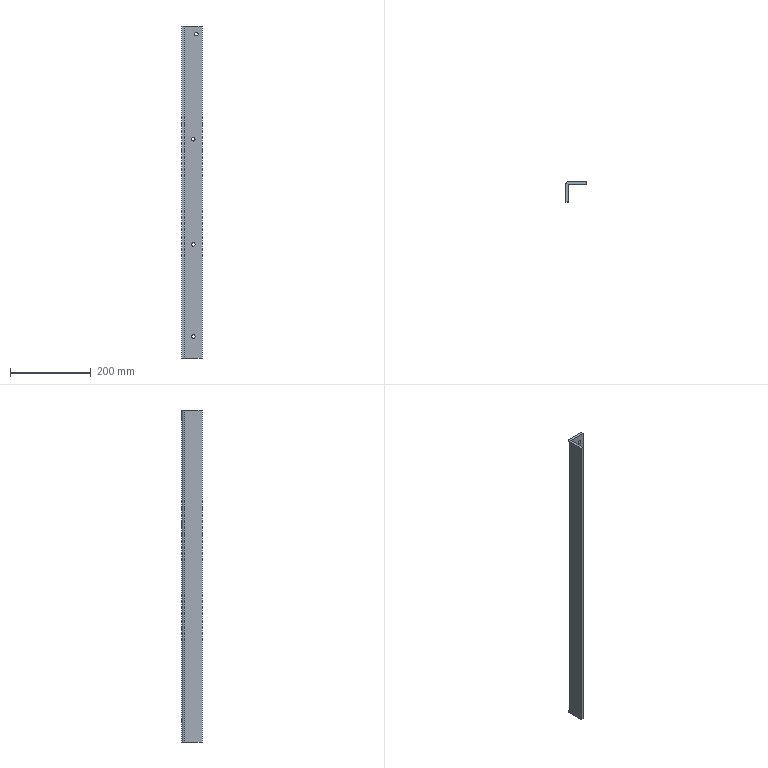Part | SolidWorks | features BaseBody 1 | 1 solid | 18 faces | box 50 x 50 x 821 mm | volume 453617 mm3 | cylinder 10 | plane 8 | commonest cylinder face diameters 9 x8 1.473 x1 13.473 x1
STEP:
#1=CARTESIAN_POINT('',(28.,50.,57.5));
#2=VERTEX_POINT('',#1);
#3=CARTESIAN_POINT('',(28.,50.,48.5));
#4=VERTEX_POINT('',#3);
#5=CARTESIAN_POINT('',(28.,50.,53.));
#6=DIRECTION('',(0.,-1.,0.));
#7=DIRECTION('',(0.,0.,-1.));
#8=AXIS2_PLACEMENT_3D('',#5,#6,#7);
#9=CIRCLE('',#8,4.5);
#10=EDGE_CURVE('',#2,#4,#9,.T.);
#11=ORIENTED_EDGE('',*,*,#10,.F.);
#12=CARTESIAN_POINT('',(28.,44.,57.5));
#13=VERTEX_POINT('',#12);
#14=CARTESIAN_POINT('',(28.,50.,57.5));
#15=DIRECTION('',(0.,-1.,0.));
#16=VECTOR('',#15,1000.);
#17=LINE('',#14,#16);
#18=EDGE_CURVE('',#2,#13,#17,.T.);
#19=ORIENTED_EDGE('',*,*,#18,.T.);
#20=CARTESIAN_POINT('',(28.,44.,48.5));
#21=VERTEX_POINT('',#20);
#22=CARTESIAN_POINT('',(28.,44.,53.));
#23=DIRECTION('',(0.,1.,0.));
#24=DIRECTION('',(0.,0.,-1.));
#25=AXIS2_PLACEMENT_3D('',#22,#23,#24);
#26=CIRCLE('',#25,4.5);
#27=EDGE_CURVE('',#21,#13,#26,.T.);
#28=ORIENTED_EDGE('',*,*,#27,.F.);
#29=CARTESIAN_POINT('',(28.,50.,48.5));
#30=DIRECTION('',(0.,-1.,0.));
#31=VECTOR('',#30,1000.);
#32=LINE('',#29,#31);
#33=EDGE_CURVE('',#4,#21,#32,.T.);
#34=ORIENTED_EDGE('',*,*,#33,.F.);
#35=EDGE_LOOP('',(#11,#19,#28,#34));
#36=FACE_OUTER_BOUND('',#35,.T.);
#37=CARTESIAN_POINT('',(28.,50.,53.));
#38=DIRECTION('',(0.,-1.,0.));
#39=DIRECTION('',(0.,0.,-1.));
#40=AXIS2_PLACEMENT_3D('',#37,#38,#39);
#41=CYLINDRICAL_SURFACE('',#40,4.5);
#42=ADVANCED_FACE('',(#36),#41,.F.);
#43=CARTESIAN_POINT('',(28.,50.,285.5));
#44=VERTEX_POINT('',#43);
#45=CARTESIAN_POINT('',(28.,50.,276.5));
#46=VERTEX_POINT('',#45);
#47=CARTESIAN_POINT('',(28.,50.,281.));
#48=DIRECTION('',(0.,-1.,0.));
#49=DIRECTION('',(0.,0.,-1.));
#50=AXIS2_PLACEMENT_3D('',#47,#48,#49);
#51=CIRCLE('',#50,4.5);
#52=EDGE_CURVE('',#44,#46,#51,.T.);
#53=ORIENTED_EDGE('',*,*,#52,.F.);
#54=CARTESIAN_POINT('',(28.,44.,285.5));
#55=VERTEX_POINT('',#54);
#56=CARTESIAN_POINT('',(28.,50.,285.5));
#57=DIRECTION('',(0.,-1.,0.));
#58=VECTOR('',#57,1000.);
#59=LINE('',#56,#58);
#60=EDGE_CURVE('',#44,#55,#59,.T.);
#61=ORIENTED_EDGE('',*,*,#60,.T.);
#62=CARTESIAN_POINT('',(28.,44.,276.5));
#63=VERTEX_POINT('',#62);
#64=CARTESIAN_POINT('',(28.,44.,281.));
#65=DIRECTION('',(0.,1.,0.));
#66=DIRECTION('',(0.,0.,-1.));
#67=AXIS2_PLACEMENT_3D('',#64,#65,#66);
#68=CIRCLE('',#67,4.5);
#69=EDGE_CURVE('',#63,#55,#68,.T.);
#70=ORIENTED_EDGE('',*,*,#69,.F.);
#71=CARTESIAN_POINT('',(28.,50.,276.5));
#72=DIRECTION('',(0.,-1.,0.));
#73=VECTOR('',#72,1000.);
#74=LINE('',#71,#73);
#75=EDGE_CURVE('',#46,#63,#74,.T.);
#76=ORIENTED_EDGE('',*,*,#75,.F.);
#77=EDGE_LOOP('',(#53,#61,#70,#76));
#78=FACE_OUTER_BOUND('',#77,.T.);
#79=CARTESIAN_POINT('',(28.,50.,281.));
#80=DIRECTION('',(0.,-1.,0.));
#81=DIRECTION('',(0.,0.,-1.));
#82=AXIS2_PLACEMENT_3D('',#79,#80,#81);
#83=CYLINDRICAL_SURFACE('',#82,4.5);
#84=ADVANCED_FACE('',(#78),#83,.F.);
#85=CARTESIAN_POINT('',(28.,50.,545.5));
#86=VERTEX_POINT('',#85);
#87=CARTESIAN_POINT('',(28.,50.,536.5));
#88=VERTEX_POINT('',#87);
#89=CARTESIAN_POINT('',(28.,50.,541.));
#90=DIRECTION('',(0.,-1.,0.));
#91=DIRECTION('',(0.,0.,-1.));
#92=AXIS2_PLACEMENT_3D('',#89,#90,#91);
#93=CIRCLE('',#92,4.5);
#94=EDGE_CURVE('',#86,#88,#93,.T.);
#95=ORIENTED_EDGE('',*,*,#94,.F.);
#96=CARTESIAN_POINT('',(28.,44.,545.5));
#97=VERTEX_POINT('',#96);
#98=CARTESIAN_POINT('',(28.,50.,545.5));
#99=DIRECTION('',(0.,-1.,0.));
#100=VECTOR('',#99,1000.);
#101=LINE('',#98,#100);
#102=EDGE_CURVE('',#86,#97,#101,.T.);
#103=ORIENTED_EDGE('',*,*,#102,.T.);
#104=CARTESIAN_POINT('',(28.,44.,536.5));
#105=VERTEX_POINT('',#104);
#106=CARTESIAN_POINT('',(28.,44.,541.));
#107=DIRECTION('',(0.,1.,0.));
#108=DIRECTION('',(0.,0.,-1.));
#109=AXIS2_PLACEMENT_3D('',#106,#107,#108);
#110=CIRCLE('',#109,4.5);
#111=EDGE_CURVE('',#105,#97,#110,.T.);
#112=ORIENTED_EDGE('',*,*,#111,.F.);
#113=CARTESIAN_POINT('',(28.,50.,536.5));
#114=DIRECTION('',(0.,-1.,0.));
#115=VECTOR('',#114,1000.);
#116=LINE('',#113,#115);
#117=EDGE_CURVE('',#88,#105,#116,.T.);
#118=ORIENTED_EDGE('',*,*,#117,.F.);
#119=EDGE_LOOP('',(#95,#103,#112,#118));
#120=FACE_OUTER_BOUND('',#119,.T.);
#121=CARTESIAN_POINT('',(28.,50.,541.));
#122=DIRECTION('',(0.,-1.,0.));
#123=DIRECTION('',(0.,0.,-1.));
#124=AXIS2_PLACEMENT_3D('',#121,#122,#123);
#125=CYLINDRICAL_SURFACE('',#124,4.5);
#126=ADVANCED_FACE('',(#120),#125,.F.);
#127=CARTESIAN_POINT('',(36.,50.,805.5));
#128=VERTEX_POINT('',#127);
#129=CARTESIAN_POINT('',(36.,50.,796.5));
#130=VERTEX_POINT('',#129);
#131=CARTESIAN_POINT('',(36.,50.,801.));
#132=DIRECTION('',(0.,-1.,0.));
#133=DIRECTION('',(0.,0.,-1.));
#134=AXIS2_PLACEMENT_3D('',#131,#132,#133);
#135=CIRCLE('',#134,4.5);
#136=EDGE_CURVE('',#128,#130,#135,.T.);
#137=ORIENTED_EDGE('',*,*,#136,.F.);
#138=CARTESIAN_POINT('',(36.,44.,805.5));
#139=VERTEX_POINT('',#138);
#140=CARTESIAN_POINT('',(36.,50.,805.5));
#141=DIRECTION('',(0.,-1.,0.));
#142=VECTOR('',#141,1000.);
#143=LINE('',#140,#142);
#144=EDGE_CURVE('',#128,#139,#143,.T.);
#145=ORIENTED_EDGE('',*,*,#144,.T.);
#146=CARTESIAN_POINT('',(36.,44.,796.5));
#147=VERTEX_POINT('',#146);
#148=CARTESIAN_POINT('',(36.,44.,801.));
#149=DIRECTION('',(0.,1.,0.));
#150=DIRECTION('',(0.,0.,-1.));
#151=AXIS2_PLACEMENT_3D('',#148,#149,#150);
#152=CIRCLE('',#151,4.5);
#153=EDGE_CURVE('',#147,#139,#152,.T.);
#154=ORIENTED_EDGE('',*,*,#153,.F.);
#155=CARTESIAN_POINT('',(36.,50.,796.5));
#156=DIRECTION('',(0.,-1.,0.));
#157=VECTOR('',#156,1000.);
#158=LINE('',#155,#157);
#159=EDGE_CURVE('',#130,#147,#158,.T.);
#160=ORIENTED_EDGE('',*,*,#159,.F.);
#161=EDGE_LOOP('',(#137,#145,#154,#160));
#162=FACE_OUTER_BOUND('',#161,.T.);
#163=CARTESIAN_POINT('',(36.,50.,801.));
#164=DIRECTION('',(0.,-1.,0.));
#165=DIRECTION('',(0.,0.,-1.));
#166=AXIS2_PLACEMENT_3D('',#163,#164,#165);
#167=CYLINDRICAL_SURFACE('',#166,4.5);
#168=ADVANCED_FACE('',(#162),#167,.F.);
#169=CARTESIAN_POINT('',(0.,0.,821.));
#170=VERTEX_POINT('',#169);
#171=CARTESIAN_POINT('',(0.,43.263,821.));
#172=VERTEX_POINT('',#171);
#173=CARTESIAN_POINT('',(0.,0.,821.));
#174=DIRECTION('',(0.,1.,0.));
#175=VECTOR('',#174,1000.);
#176=LINE('',#173,#175);
#177=EDGE_CURVE('',#170,#172,#176,.T.);
#178=ORIENTED_EDGE('',*,*,#177,.T.);
#179=CARTESIAN_POINT('',(0.,43.263,0.));
#180=VERTEX_POINT('',#179);
#181=CARTESIAN_POINT('',(0.,43.263,821.));
#182=DIRECTION('',(0.,0.,-1.));
#183=VECTOR('',#182,1000.);
#184=LINE('',#181,#183);
#185=EDGE_CURVE('',#172,#180,#184,.T.);
#186=ORIENTED_EDGE('',*,*,#185,.T.);
#187=CARTESIAN_POINT('',(0.,0.,0.));
#188=VERTEX_POINT('',#187);
#189=CARTESIAN_POINT('',(0.,0.,0.));
#190=DIRECTION('',(0.,-1.,0.));
#191=VECTOR('',#190,1000.);
#192=LINE('',#189,#191);
#193=EDGE_CURVE('',#180,#188,#192,.T.);
#194=ORIENTED_EDGE('',*,*,#193,.T.);
#195=CARTESIAN_POINT('',(0.,0.,821.));
#196=DIRECTION('',(0.,0.,1.));
#197=VECTOR('',#196,1000.);
#198=LINE('',#195,#197);
#199=EDGE_CURVE('',#188,#170,#198,.T.);
#200=ORIENTED_EDGE('',*,*,#199,.T.);
#201=EDGE_LOOP('',(#178,#186,#194,#200));
#202=FACE_OUTER_BOUND('',#201,.T.);
#203=CARTESIAN_POINT('',(0.,0.,821.));
#204=DIRECTION('',(-1.,0.,0.));
#205=DIRECTION('',(0.,0.,1.));
#206=AXIS2_PLACEMENT_3D('',#203,#204,#205);
#207=PLANE('',#206);
#208=ADVANCED_FACE('',(#202),#207,.T.);
#209=CARTESIAN_POINT('',(6.737,50.,821.));
#210=VERTEX_POINT('',#209);
#211=CARTESIAN_POINT('',(6.737,43.263,821.));
#212=DIRECTION('',(0.,0.,-1.));
#213=DIRECTION('',(-1.,0.,0.));
#214=AXIS2_PLACEMENT_3D('',#211,#212,#213);
#215=CIRCLE('',#214,6.737);
#216=EDGE_CURVE('',#172,#210,#215,.T.);
#217=ORIENTED_EDGE('',*,*,#216,.T.);
#218=CARTESIAN_POINT('',(6.737,50.,0.));
#219=VERTEX_POINT('',#218);
#220=CARTESIAN_POINT('',(6.737,50.,821.));
#221=DIRECTION('',(0.,0.,-1.));
#222=VECTOR('',#221,1000.);
#223=LINE('',#220,#222);
#224=EDGE_CURVE('',#210,#219,#223,.T.);
#225=ORIENTED_EDGE('',*,*,#224,.T.);
#226=CARTESIAN_POINT('',(6.737,43.263,0.));
#227=DIRECTION('',(0.,0.,1.));
#228=DIRECTION('',(-1.,0.,0.));
#229=AXIS2_PLACEMENT_3D('',#226,#227,#228);
#230=CIRCLE('',#229,6.737);
#231=EDGE_CURVE('',#219,#180,#230,.T.);
#232=ORIENTED_EDGE('',*,*,#231,.T.);
#233=ORIENTED_EDGE('',*,*,#185,.F.);
#234=EDGE_LOOP('',(#217,#225,#232,#233));
#235=FACE_OUTER_BOUND('',#234,.T.);
#236=CARTESIAN_POINT('',(6.737,43.263,821.));
#237=DIRECTION('',(0.,0.,-1.));
#238=DIRECTION('',(-1.,0.,0.));
#239=AXIS2_PLACEMENT_3D('',#236,#237,#238);
#240=CYLINDRICAL_SURFACE('',#239,6.737);
#241=ADVANCED_FACE('',(#235),#240,.T.);
#242=ORIENTED_EDGE('',*,*,#177,.F.);
#243=CARTESIAN_POINT('',(6.,0.,821.));
#244=VERTEX_POINT('',#243);
#245=CARTESIAN_POINT('',(6.737,0.,821.));
#246=DIRECTION('',(1.,0.,0.));
#247=VECTOR('',#246,1000.);
#248=LINE('',#245,#247);
#249=EDGE_CURVE('',#170,#244,#248,.T.);
#250=ORIENTED_EDGE('',*,*,#249,.T.);
#251=CARTESIAN_POINT('',(6.,43.263,821.));
#252=VERTEX_POINT('',#251);
#253=CARTESIAN_POINT('',(6.,43.263,821.));
#254=DIRECTION('',(0.,1.,0.));
#255=VECTOR('',#254,1000.);
#256=LINE('',#253,#255);
#257=EDGE_CURVE('',#244,#252,#256,.T.);
#258=ORIENTED_EDGE('',*,*,#257,.T.);
#259=CARTESIAN_POINT('',(6.737,44.,821.));
#260=VERTEX_POINT('',#259);
#261=CARTESIAN_POINT('',(6.737,43.263,821.));
#262=DIRECTION('',(0.,0.,-1.));
#263=DIRECTION('',(-1.,0.,0.));
#264=AXIS2_PLACEMENT_3D('',#261,#262,#263);
#265=CIRCLE('',#264,0.7366);
#266=EDGE_CURVE('',#252,#260,#265,.T.);
#267=ORIENTED_EDGE('',*,*,#266,.T.);
#268=CARTESIAN_POINT('',(50.,44.,821.));
#269=VERTEX_POINT('',#268);
#270=CARTESIAN_POINT('',(6.,44.,821.));
#271=DIRECTION('',(1.,0.,0.));
#272=VECTOR('',#271,1000.);
#273=LINE('',#270,#272);
#274=EDGE_CURVE('',#260,#269,#273,.T.);
#275=ORIENTED_EDGE('',*,*,#274,.T.);
#276=CARTESIAN_POINT('',(50.,50.,821.));
#277=VERTEX_POINT('',#276);
#278=CARTESIAN_POINT('',(50.,50.,821.));
#279=DIRECTION('',(0.,-1.,0.));
#280=VECTOR('',#279,1000.);
#281=LINE('',#278,#280);
#282=EDGE_CURVE('',#277,#269,#281,.T.);
#283=ORIENTED_EDGE('',*,*,#282,.F.);
#284=CARTESIAN_POINT('',(0.,50.,821.));
#285=DIRECTION('',(1.,0.,0.));
#286=VECTOR('',#285,1000.);
#287=LINE('',#284,#286);
#288=EDGE_CURVE('',#210,#277,#287,.T.);
#289=ORIENTED_EDGE('',*,*,#288,.F.);
#290=ORIENTED_EDGE('',*,*,#216,.F.);
#291=EDGE_LOOP('',(#242,#250,#258,#267,#275,#283,#289,#290));
#292=FACE_OUTER_BOUND('',#291,.T.);
#293=CARTESIAN_POINT('',(6.737,43.263,821.));
#294=DIRECTION('',(0.,0.,1.));
#295=DIRECTION('',(1.,0.,0.));
#296=AXIS2_PLACEMENT_3D('',#293,#294,#295);
#297=PLANE('',#296);
#298=ADVANCED_FACE('',(#292),#297,.T.);
#299=ORIENTED_EDGE('',*,*,#249,.F.);
#300=ORIENTED_EDGE('',*,*,#199,.F.);
#301=CARTESIAN_POINT('',(6.,0.,0.));
#302=VERTEX_POINT('',#301);
#303=CARTESIAN_POINT('',(6.,0.,0.));
#304=DIRECTION('',(1.,0.,0.));
#305=VECTOR('',#304,1000.);
#306=LINE('',#303,#305);
#307=EDGE_CURVE('',#188,#302,#306,.T.);
#308=ORIENTED_EDGE('',*,*,#307,.T.);
#309=CARTESIAN_POINT('',(6.,0.,821.));
#310=DIRECTION('',(0.,0.,1.));
#311=VECTOR('',#310,1000.);
#312=LINE('',#309,#311);
#313=EDGE_CURVE('',#302,#244,#312,.T.);
#314=ORIENTED_EDGE('',*,*,#313,.T.);
#315=EDGE_LOOP('',(#299,#300,#308,#314));
#316=FACE_OUTER_BOUND('',#315,.T.);
#317=CARTESIAN_POINT('',(6.,0.,821.));
#318=DIRECTION('',(0.,-1.,0.));
#319=DIRECTION('',(0.,0.,-1.));
#320=AXIS2_PLACEMENT_3D('',#317,#318,#319);
#321=PLANE('',#320);
#322=ADVANCED_FACE('',(#316),#321,.T.);
#323=CARTESIAN_POINT('',(6.,43.263,0.));
#324=VERTEX_POINT('',#323);
#325=CARTESIAN_POINT('',(6.,44.,0.));
#326=DIRECTION('',(0.,-1.,0.));
#327=VECTOR('',#326,1000.);
#328=LINE('',#325,#327);
#329=EDGE_CURVE('',#324,#302,#328,.T.);
#330=ORIENTED_EDGE('',*,*,#329,.T.);
#331=ORIENTED_EDGE('',*,*,#307,.F.);
#332=ORIENTED_EDGE('',*,*,#193,.F.);
#333=ORIENTED_EDGE('',*,*,#231,.F.);
#334=CARTESIAN_POINT('',(50.,50.,0.));
#335=VERTEX_POINT('',#334);
#336=CARTESIAN_POINT('',(0.,50.,0.));
#337=DIRECTION('',(-1.,0.,0.));
#338=VECTOR('',#337,1000.);
#339=LINE('',#336,#338);
#340=EDGE_CURVE('',#335,#219,#339,.T.);
#341=ORIENTED_EDGE('',*,*,#340,.F.);
#342=CARTESIAN_POINT('',(50.,44.,0.));
#343=VERTEX_POINT('',#342);
#344=CARTESIAN_POINT('',(50.,50.,0.));
#345=DIRECTION('',(0.,1.,0.));
#346=VECTOR('',#345,1000.);
#347=LINE('',#344,#346);
#348=EDGE_CURVE('',#343,#335,#347,.T.);
#349=ORIENTED_EDGE('',*,*,#348,.F.);
#350=CARTESIAN_POINT('',(6.737,44.,0.));
#351=VERTEX_POINT('',#350);
#352=CARTESIAN_POINT('',(6.737,44.,0.));
#353=DIRECTION('',(1.,0.,0.));
#354=VECTOR('',#353,1000.);
#355=LINE('',#352,#354);
#356=EDGE_CURVE('',#351,#343,#355,.T.);
#357=ORIENTED_EDGE('',*,*,#356,.F.);
#358=CARTESIAN_POINT('',(6.737,43.263,0.));
#359=DIRECTION('',(0.,0.,1.));
#360=DIRECTION('',(-1.,0.,0.));
#361=AXIS2_PLACEMENT_3D('',#358,#359,#360);
#362=CIRCLE('',#361,0.7366);
#363=EDGE_CURVE('',#351,#324,#362,.T.);
#364=ORIENTED_EDGE('',*,*,#363,.T.);
#365=EDGE_LOOP('',(#330,#331,#332,#333,#341,#349,#357,#364));
#366=FACE_OUTER_BOUND('',#365,.T.);
#367=CARTESIAN_POINT('',(6.737,44.,0.));
#368=DIRECTION('',(0.,0.,-1.));
#369=DIRECTION('',(-1.,0.,0.));
#370=AXIS2_PLACEMENT_3D('',#367,#368,#369);
#371=PLANE('',#370);
#372=ADVANCED_FACE('',(#366),#371,.T.);
#373=ORIENTED_EDGE('',*,*,#288,.T.);
#374=CARTESIAN_POINT('',(50.,50.,821.));
#375=DIRECTION('',(0.,0.,-1.));
#376=VECTOR('',#375,1000.);
#377=LINE('',#374,#376);
#378=EDGE_CURVE('',#277,#335,#377,.T.);
#379=ORIENTED_EDGE('',*,*,#378,.T.);
#380=ORIENTED_EDGE('',*,*,#340,.T.);
#381=ORIENTED_EDGE('',*,*,#224,.F.);
#382=EDGE_LOOP('',(#373,#379,#380,#381));
#383=FACE_OUTER_BOUND('',#382,.T.);
#384=CARTESIAN_POINT('',(28.,50.,53.));
#385=DIRECTION('',(0.,-1.,0.));
#386=DIRECTION('',(0.,0.,-1.));
#387=AXIS2_PLACEMENT_3D('',#384,#385,#386);
#388=CIRCLE('',#387,4.5);
#389=EDGE_CURVE('',#4,#2,#388,.T.);
#390=ORIENTED_EDGE('',*,*,#389,.T.);
#391=ORIENTED_EDGE('',*,*,#10,.T.);
#392=EDGE_LOOP('',(#390,#391));
#393=FACE_BOUND('',#392,.T.);
#394=CARTESIAN_POINT('',(28.,50.,281.));
#395=DIRECTION('',(0.,-1.,0.));
#396=DIRECTION('',(0.,0.,-1.));
#397=AXIS2_PLACEMENT_3D('',#394,#395,#396);
#398=CIRCLE('',#397,4.5);
#399=EDGE_CURVE('',#46,#44,#398,.T.);
#400=ORIENTED_EDGE('',*,*,#399,.T.);
#401=ORIENTED_EDGE('',*,*,#52,.T.);
#402=EDGE_LOOP('',(#400,#401));
#403=FACE_BOUND('',#402,.T.);
#404=CARTESIAN_POINT('',(28.,50.,541.));
#405=DIRECTION('',(0.,-1.,0.));
#406=DIRECTION('',(0.,0.,-1.));
#407=AXIS2_PLACEMENT_3D('',#404,#405,#406);
#408=CIRCLE('',#407,4.5);
#409=EDGE_CURVE('',#88,#86,#408,.T.);
#410=ORIENTED_EDGE('',*,*,#409,.T.);
#411=ORIENTED_EDGE('',*,*,#94,.T.);
#412=EDGE_LOOP('',(#410,#411));
#413=FACE_BOUND('',#412,.T.);
#414=CARTESIAN_POINT('',(36.,50.,801.));
#415=DIRECTION('',(0.,-1.,0.));
#416=DIRECTION('',(0.,0.,-1.));
#417=AXIS2_PLACEMENT_3D('',#414,#415,#416);
#418=CIRCLE('',#417,4.5);
#419=EDGE_CURVE('',#130,#128,#418,.T.);
#420=ORIENTED_EDGE('',*,*,#419,.T.);
#421=ORIENTED_EDGE('',*,*,#136,.T.);
#422=EDGE_LOOP('',(#420,#421));
#423=FACE_BOUND('',#422,.T.);
#424=CARTESIAN_POINT('',(0.,50.,821.));
#425=DIRECTION('',(0.,1.,0.));
#426=DIRECTION('',(0.,0.,1.));
#427=AXIS2_PLACEMENT_3D('',#424,#425,#426);
#428=PLANE('',#427);
#429=ADVANCED_FACE('',(#383,#393,#403,#413,#423),#428,.T.);
#430=CARTESIAN_POINT('',(6.,43.263,821.));
#431=DIRECTION('',(0.,0.,-1.));
#432=VECTOR('',#431,1000.);
#433=LINE('',#430,#432);
#434=EDGE_CURVE('',#252,#324,#433,.T.);
#435=ORIENTED_EDGE('',*,*,#434,.F.);
#436=ORIENTED_EDGE('',*,*,#257,.F.);
#437=ORIENTED_EDGE('',*,*,#313,.F.);
#438=ORIENTED_EDGE('',*,*,#329,.F.);
#439=EDGE_LOOP('',(#435,#436,#437,#438));
#440=FACE_OUTER_BOUND('',#439,.T.);
#441=CARTESIAN_POINT('',(6.,0.,821.));
#442=DIRECTION('',(-1.,0.,0.));
#443=DIRECTION('',(0.,0.,1.));
#444=AXIS2_PLACEMENT_3D('',#441,#442,#443);
#445=PLANE('',#444);
#446=ADVANCED_FACE('',(#440),#445,.F.);
#447=ORIENTED_EDGE('',*,*,#282,.T.);
#448=CARTESIAN_POINT('',(50.,44.,821.));
#449=DIRECTION('',(0.,0.,-1.));
#450=VECTOR('',#449,1000.);
#451=LINE('',#448,#450);
#452=EDGE_CURVE('',#269,#343,#451,.T.);
#453=ORIENTED_EDGE('',*,*,#452,.T.);
#454=ORIENTED_EDGE('',*,*,#348,.T.);
#455=ORIENTED_EDGE('',*,*,#378,.F.);
#456=EDGE_LOOP('',(#447,#453,#454,#455));
#457=FACE_OUTER_BOUND('',#456,.T.);
#458=CARTESIAN_POINT('',(50.,50.,821.));
#459=DIRECTION('',(1.,0.,0.));
#460=DIRECTION('',(0.,0.,-1.));
#461=AXIS2_PLACEMENT_3D('',#458,#459,#460);
#462=PLANE('',#461);
#463=ADVANCED_FACE('',(#457),#462,.T.);
#464=ORIENTED_EDGE('',*,*,#18,.F.);
#465=ORIENTED_EDGE('',*,*,#389,.F.);
#466=ORIENTED_EDGE('',*,*,#33,.T.);
#467=CARTESIAN_POINT('',(28.,44.,53.));
#468=DIRECTION('',(0.,1.,0.));
#469=DIRECTION('',(0.,0.,-1.));
#470=AXIS2_PLACEMENT_3D('',#467,#468,#469);
#471=CIRCLE('',#470,4.5);
#472=EDGE_CURVE('',#13,#21,#471,.T.);
#473=ORIENTED_EDGE('',*,*,#472,.F.);
#474=EDGE_LOOP('',(#464,#465,#466,#473));
#475=FACE_OUTER_BOUND('',#474,.T.);
#476=CARTESIAN_POINT('',(28.,50.,53.));
#477=DIRECTION('',(0.,-1.,0.));
#478=DIRECTION('',(0.,0.,-1.));
#479=AXIS2_PLACEMENT_3D('',#476,#477,#478);
#480=CYLINDRICAL_SURFACE('',#479,4.5);
#481=ADVANCED_FACE('',(#475),#480,.F.);
#482=ORIENTED_EDGE('',*,*,#60,.F.);
#483=ORIENTED_EDGE('',*,*,#399,.F.);
#484=ORIENTED_EDGE('',*,*,#75,.T.);
#485=CARTESIAN_POINT('',(28.,44.,281.));
#486=DIRECTION('',(0.,1.,0.));
#487=DIRECTION('',(0.,0.,-1.));
#488=AXIS2_PLACEMENT_3D('',#485,#486,#487);
#489=CIRCLE('',#488,4.5);
#490=EDGE_CURVE('',#55,#63,#489,.T.);
#491=ORIENTED_EDGE('',*,*,#490,.F.);
#492=EDGE_LOOP('',(#482,#483,#484,#491));
#493=FACE_OUTER_BOUND('',#492,.T.);
#494=CARTESIAN_POINT('',(28.,50.,281.));
#495=DIRECTION('',(0.,-1.,0.));
#496=DIRECTION('',(0.,0.,-1.));
#497=AXIS2_PLACEMENT_3D('',#494,#495,#496);
#498=CYLINDRICAL_SURFACE('',#497,4.5);
#499=ADVANCED_FACE('',(#493),#498,.F.);
#500=ORIENTED_EDGE('',*,*,#102,.F.);
#501=ORIENTED_EDGE('',*,*,#409,.F.);
#502=ORIENTED_EDGE('',*,*,#117,.T.);
#503=CARTESIAN_POINT('',(28.,44.,541.));
#504=DIRECTION('',(0.,1.,0.));
#505=DIRECTION('',(0.,0.,-1.));
#506=AXIS2_PLACEMENT_3D('',#503,#504,#505);
#507=CIRCLE('',#506,4.5);
#508=EDGE_CURVE('',#97,#105,#507,.T.);
#509=ORIENTED_EDGE('',*,*,#508,.F.);
#510=EDGE_LOOP('',(#500,#501,#502,#509));
#511=FACE_OUTER_BOUND('',#510,.T.);
#512=CARTESIAN_POINT('',(28.,50.,541.));
#513=DIRECTION('',(0.,-1.,0.));
#514=DIRECTION('',(0.,0.,-1.));
#515=AXIS2_PLACEMENT_3D('',#512,#513,#514);
#516=CYLINDRICAL_SURFACE('',#515,4.5);
#517=ADVANCED_FACE('',(#511),#516,.F.);
#518=ORIENTED_EDGE('',*,*,#144,.F.);
#519=ORIENTED_EDGE('',*,*,#419,.F.);
#520=ORIENTED_EDGE('',*,*,#159,.T.);
#521=CARTESIAN_POINT('',(36.,44.,801.));
#522=DIRECTION('',(0.,1.,0.));
#523=DIRECTION('',(0.,0.,-1.));
#524=AXIS2_PLACEMENT_3D('',#521,#522,#523);
#525=CIRCLE('',#524,4.5);
#526=EDGE_CURVE('',#139,#147,#525,.T.);
#527=ORIENTED_EDGE('',*,*,#526,.F.);
#528=EDGE_LOOP('',(#518,#519,#520,#527));
#529=FACE_OUTER_BOUND('',#528,.T.);
#530=CARTESIAN_POINT('',(36.,50.,801.));
#531=DIRECTION('',(0.,-1.,0.));
#532=DIRECTION('',(0.,0.,-1.));
#533=AXIS2_PLACEMENT_3D('',#530,#531,#532);
#534=CYLINDRICAL_SURFACE('',#533,4.5);
#535=ADVANCED_FACE('',(#529),#534,.F.);
#536=CARTESIAN_POINT('',(6.737,44.,821.));
#537=DIRECTION('',(0.,0.,-1.));
#538=VECTOR('',#537,1000.);
#539=LINE('',#536,#538);
#540=EDGE_CURVE('',#260,#351,#539,.T.);
#541=ORIENTED_EDGE('',*,*,#540,.F.);
#542=ORIENTED_EDGE('',*,*,#266,.F.);
#543=ORIENTED_EDGE('',*,*,#434,.T.);
#544=ORIENTED_EDGE('',*,*,#363,.F.);
#545=EDGE_LOOP('',(#541,#542,#543,#544));
#546=FACE_OUTER_BOUND('',#545,.T.);
#547=CARTESIAN_POINT('',(6.737,43.263,821.));
#548=DIRECTION('',(0.,0.,-1.));
#549=DIRECTION('',(-1.,0.,0.));
#550=AXIS2_PLACEMENT_3D('',#547,#548,#549);
#551=CYLINDRICAL_SURFACE('',#550,0.7366);
#552=ADVANCED_FACE('',(#546),#551,.F.);
#553=ORIENTED_EDGE('',*,*,#452,.F.);
#554=ORIENTED_EDGE('',*,*,#274,.F.);
#555=ORIENTED_EDGE('',*,*,#540,.T.);
#556=ORIENTED_EDGE('',*,*,#356,.T.);
#557=EDGE_LOOP('',(#553,#554,#555,#556));
#558=FACE_OUTER_BOUND('',#557,.T.);
#559=ORIENTED_EDGE('',*,*,#27,.T.);
#560=ORIENTED_EDGE('',*,*,#472,.T.);
#561=EDGE_LOOP('',(#559,#560));
#562=FACE_BOUND('',#561,.T.);
#563=ORIENTED_EDGE('',*,*,#69,.T.);
#564=ORIENTED_EDGE('',*,*,#490,.T.);
#565=EDGE_LOOP('',(#563,#564));
#566=FACE_BOUND('',#565,.T.);
#567=ORIENTED_EDGE('',*,*,#111,.T.);
#568=ORIENTED_EDGE('',*,*,#508,.T.);
#569=EDGE_LOOP('',(#567,#568));
#570=FACE_BOUND('',#569,.T.);
#571=ORIENTED_EDGE('',*,*,#153,.T.);
#572=ORIENTED_EDGE('',*,*,#526,.T.);
#573=EDGE_LOOP('',(#571,#572));
#574=FACE_BOUND('',#573,.T.);
#575=CARTESIAN_POINT('',(0.,44.,821.));
#576=DIRECTION('',(0.,1.,0.));
#577=DIRECTION('',(0.,0.,1.));
#578=AXIS2_PLACEMENT_3D('',#575,#576,#577);
#579=PLANE('',#578);
#580=ADVANCED_FACE('',(#558,#562,#566,#570,#574),#579,.F.);
#581=CLOSED_SHELL('',(#42,#84,#126,#168,#208,#241,#298,#322,#372,#429,#446,#463,#481,#499,#517,#535,#552,#580));
#582=MANIFOLD_SOLID_BREP('',#581);
#583=CARTESIAN_POINT('',(0.,0.,0.));
#584=DIRECTION('',(0.,0.,1.));
#585=DIRECTION('',(1.,0.,0.));
#586=AXIS2_PLACEMENT_3D('',#583,#584,#585);
#587=(LENGTH_UNIT()NAMED_UNIT(*)SI_UNIT(.MILLI.,.METRE.));
#588=UNCERTAINTY_MEASURE_WITH_UNIT(LENGTH_MEASURE(0.00001),#587,'','');
#589=(NAMED_UNIT(*)PLANE_ANGLE_UNIT()SI_UNIT($,.RADIAN.));
#590=(NAMED_UNIT(*)SI_UNIT($,.STERADIAN.)SOLID_ANGLE_UNIT());
#591=(GEOMETRIC_REPRESENTATION_CONTEXT(3)GLOBAL_UNCERTAINTY_ASSIGNED_CONTEXT((#588))GLOBAL_UNIT_ASSIGNED_CONTEXT((#587,#589,#590))REPRESENTATION_CONTEXT('',''));
#592=ADVANCED_BREP_SHAPE_REPRESENTATION('',(#582,#586),#591);